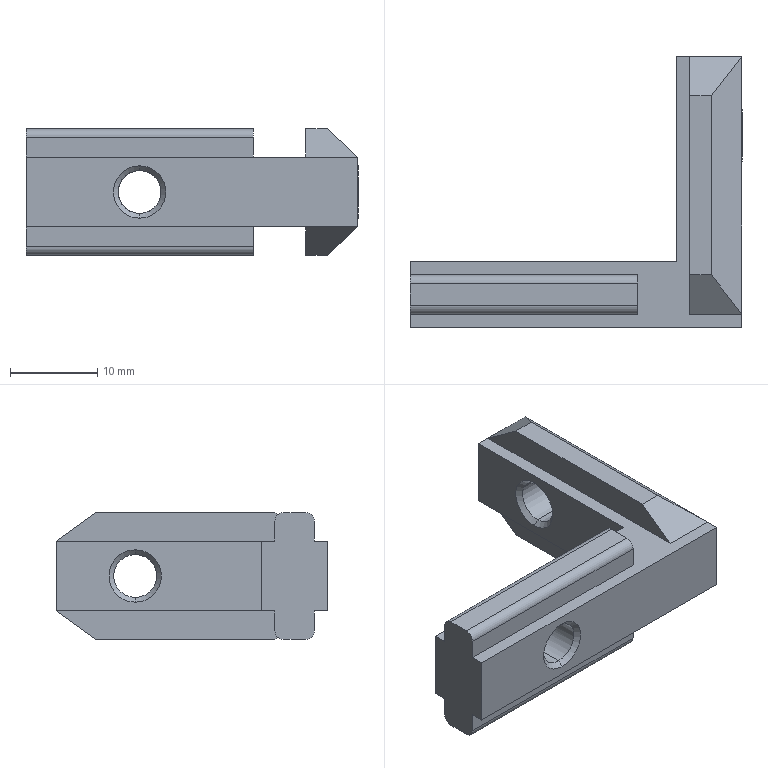Part | SolidWorks | features BaseBody 1 | 1 solid | 42 faces | box 38 x 31 x 14.5 mm | volume 4841 mm3 | plane 26 | cone 8 | cylinder 8 | commonest cylinder face diameters 2 x4 4.917 x4
STEP:
#1=CARTESIAN_POINT('',(12.,0.5415,2.458));
#2=VERTEX_POINT('',#1);
#3=CARTESIAN_POINT('',(12.,0.5415,-2.458));
#4=VERTEX_POINT('',#3);
#5=CARTESIAN_POINT('',(12.,0.5415,0.));
#6=DIRECTION('',(0.,-1.,0.));
#7=DIRECTION('',(0.,0.,-1.));
#8=AXIS2_PLACEMENT_3D('',#5,#6,#7);
#9=CIRCLE('',#8,2.458);
#10=EDGE_CURVE('',#2,#4,#9,.T.);
#11=ORIENTED_EDGE('',*,*,#10,.F.);
#12=CARTESIAN_POINT('',(12.,0.,3.));
#13=VERTEX_POINT('',#12);
#14=CARTESIAN_POINT('',(12.,0.,3.));
#15=DIRECTION('',(0.,-0.7071,0.7071));
#16=VECTOR('',#15,1000.);
#17=LINE('',#14,#16);
#18=EDGE_CURVE('',#2,#13,#17,.T.);
#19=ORIENTED_EDGE('',*,*,#18,.T.);
#20=CARTESIAN_POINT('',(12.,0.,-3.));
#21=VERTEX_POINT('',#20);
#22=CARTESIAN_POINT('',(12.,0.,0.));
#23=DIRECTION('',(0.,-1.,0.));
#24=DIRECTION('',(0.,0.,-1.));
#25=AXIS2_PLACEMENT_3D('',#22,#23,#24);
#26=CIRCLE('',#25,3.);
#27=EDGE_CURVE('',#13,#21,#26,.T.);
#28=ORIENTED_EDGE('',*,*,#27,.T.);
#29=CARTESIAN_POINT('',(12.,0.,-3.));
#30=DIRECTION('',(0.,-0.7071,-0.7071));
#31=VECTOR('',#30,1000.);
#32=LINE('',#29,#31);
#33=EDGE_CURVE('',#4,#21,#32,.T.);
#34=ORIENTED_EDGE('',*,*,#33,.F.);
#35=EDGE_LOOP('',(#11,#19,#28,#34));
#36=FACE_OUTER_BOUND('',#35,.T.);
#37=CARTESIAN_POINT('',(12.,0.,0.));
#38=DIRECTION('',(0.,-1.,0.));
#39=DIRECTION('',(0.,0.,-1.));
#40=AXIS2_PLACEMENT_3D('',#37,#38,#39);
#41=CONICAL_SURFACE('',#40,3.,0.7854);
#42=ADVANCED_FACE('',(#36),#41,.F.);
#43=CARTESIAN_POINT('',(36.458,22.,2.458));
#44=VERTEX_POINT('',#43);
#45=CARTESIAN_POINT('',(36.458,22.,-2.458));
#46=VERTEX_POINT('',#45);
#47=CARTESIAN_POINT('',(36.458,22.,0.));
#48=DIRECTION('',(1.,0.,0.));
#49=DIRECTION('',(0.,0.,-1.));
#50=AXIS2_PLACEMENT_3D('',#47,#48,#49);
#51=CIRCLE('',#50,2.458);
#52=EDGE_CURVE('',#44,#46,#51,.T.);
#53=ORIENTED_EDGE('',*,*,#52,.F.);
#54=CARTESIAN_POINT('',(37.,22.,3.));
#55=VERTEX_POINT('',#54);
#56=CARTESIAN_POINT('',(37.,22.,3.));
#57=DIRECTION('',(0.7071,0.,0.7071));
#58=VECTOR('',#57,1000.);
#59=LINE('',#56,#58);
#60=EDGE_CURVE('',#44,#55,#59,.T.);
#61=ORIENTED_EDGE('',*,*,#60,.T.);
#62=CARTESIAN_POINT('',(37.,22.,-3.));
#63=VERTEX_POINT('',#62);
#64=CARTESIAN_POINT('',(37.,22.,0.));
#65=DIRECTION('',(1.,0.,0.));
#66=DIRECTION('',(0.,0.,-1.));
#67=AXIS2_PLACEMENT_3D('',#64,#65,#66);
#68=CIRCLE('',#67,3.);
#69=EDGE_CURVE('',#55,#63,#68,.T.);
#70=ORIENTED_EDGE('',*,*,#69,.T.);
#71=CARTESIAN_POINT('',(37.,22.,-3.));
#72=DIRECTION('',(0.7071,0.,-0.7071));
#73=VECTOR('',#72,1000.);
#74=LINE('',#71,#73);
#75=EDGE_CURVE('',#46,#63,#74,.T.);
#76=ORIENTED_EDGE('',*,*,#75,.F.);
#77=EDGE_LOOP('',(#53,#61,#70,#76));
#78=FACE_OUTER_BOUND('',#77,.T.);
#79=CARTESIAN_POINT('',(37.,22.,0.));
#80=DIRECTION('',(1.,0.,0.));
#81=DIRECTION('',(0.,0.,-1.));
#82=AXIS2_PLACEMENT_3D('',#79,#80,#81);
#83=CONICAL_SURFACE('',#82,3.,0.7854);
#84=ADVANCED_FACE('',(#78),#83,.F.);
#85=ORIENTED_EDGE('',*,*,#10,.T.);
#86=CARTESIAN_POINT('',(12.,6.958,-2.458));
#87=VERTEX_POINT('',#86);
#88=CARTESIAN_POINT('',(12.,0.,-2.458));
#89=DIRECTION('',(0.,1.,0.));
#90=VECTOR('',#89,1000.);
#91=LINE('',#88,#90);
#92=EDGE_CURVE('',#4,#87,#91,.T.);
#93=ORIENTED_EDGE('',*,*,#92,.T.);
#94=CARTESIAN_POINT('',(9.542,6.958,0.));
#95=VERTEX_POINT('',#94);
#96=CARTESIAN_POINT('',(12.,6.958,0.));
#97=DIRECTION('',(0.,-1.,0.));
#98=DIRECTION('',(0.,0.,1.));
#99=AXIS2_PLACEMENT_3D('',#96,#97,#98);
#100=CIRCLE('',#99,2.458);
#101=EDGE_CURVE('',#95,#87,#100,.T.);
#102=ORIENTED_EDGE('',*,*,#101,.F.);
#103=CARTESIAN_POINT('',(12.,6.958,2.458));
#104=VERTEX_POINT('',#103);
#105=CARTESIAN_POINT('',(12.,6.958,0.));
#106=DIRECTION('',(0.,-1.,0.));
#107=DIRECTION('',(0.,0.,1.));
#108=AXIS2_PLACEMENT_3D('',#105,#106,#107);
#109=CIRCLE('',#108,2.458);
#110=EDGE_CURVE('',#104,#95,#109,.T.);
#111=ORIENTED_EDGE('',*,*,#110,.F.);
#112=CARTESIAN_POINT('',(12.,0.,2.458));
#113=DIRECTION('',(0.,1.,0.));
#114=VECTOR('',#113,1000.);
#115=LINE('',#112,#114);
#116=EDGE_CURVE('',#2,#104,#115,.T.);
#117=ORIENTED_EDGE('',*,*,#116,.F.);
#118=EDGE_LOOP('',(#85,#93,#102,#111,#117));
#119=FACE_OUTER_BOUND('',#118,.T.);
#120=CARTESIAN_POINT('',(12.,0.,0.));
#121=DIRECTION('',(0.,1.,0.));
#122=DIRECTION('',(0.,0.,1.));
#123=AXIS2_PLACEMENT_3D('',#120,#121,#122);
#124=CYLINDRICAL_SURFACE('',#123,2.458);
#125=ADVANCED_FACE('',(#119),#124,.F.);
#126=ORIENTED_EDGE('',*,*,#101,.T.);
#127=CARTESIAN_POINT('',(14.458,6.958,0.));
#128=VERTEX_POINT('',#127);
#129=CARTESIAN_POINT('',(12.,6.958,0.));
#130=DIRECTION('',(0.,-1.,0.));
#131=DIRECTION('',(0.,0.,1.));
#132=AXIS2_PLACEMENT_3D('',#129,#130,#131);
#133=CIRCLE('',#132,2.458);
#134=EDGE_CURVE('',#87,#128,#133,.T.);
#135=ORIENTED_EDGE('',*,*,#134,.T.);
#136=CARTESIAN_POINT('',(15.,7.5,0.));
#137=VERTEX_POINT('',#136);
#138=CARTESIAN_POINT('',(15.,7.5,0.));
#139=DIRECTION('',(0.7071,0.7071,0.));
#140=VECTOR('',#139,1000.);
#141=LINE('',#138,#140);
#142=EDGE_CURVE('',#128,#137,#141,.T.);
#143=ORIENTED_EDGE('',*,*,#142,.T.);
#144=CARTESIAN_POINT('',(9.,7.5,0.));
#145=VERTEX_POINT('',#144);
#146=CARTESIAN_POINT('',(12.,7.5,0.));
#147=DIRECTION('',(0.,1.,0.));
#148=DIRECTION('',(-1.,0.,0.));
#149=AXIS2_PLACEMENT_3D('',#146,#147,#148);
#150=CIRCLE('',#149,3.);
#151=EDGE_CURVE('',#137,#145,#150,.T.);
#152=ORIENTED_EDGE('',*,*,#151,.T.);
#153=CARTESIAN_POINT('',(9.,7.5,0.));
#154=DIRECTION('',(-0.7071,0.7071,0.));
#155=VECTOR('',#154,1000.);
#156=LINE('',#153,#155);
#157=EDGE_CURVE('',#95,#145,#156,.T.);
#158=ORIENTED_EDGE('',*,*,#157,.F.);
#159=EDGE_LOOP('',(#126,#135,#143,#152,#158));
#160=FACE_OUTER_BOUND('',#159,.T.);
#161=CARTESIAN_POINT('',(12.,7.5,0.));
#162=DIRECTION('',(0.,1.,0.));
#163=DIRECTION('',(-1.,0.,0.));
#164=AXIS2_PLACEMENT_3D('',#161,#162,#163);
#165=CONICAL_SURFACE('',#164,3.,0.7854);
#166=ADVANCED_FACE('',(#160),#165,.F.);
#167=CARTESIAN_POINT('',(30.041,22.,-2.458));
#168=VERTEX_POINT('',#167);
#169=CARTESIAN_POINT('',(30.041,22.,2.458));
#170=VERTEX_POINT('',#169);
#171=CARTESIAN_POINT('',(30.041,22.,0.));
#172=DIRECTION('',(-1.,0.,0.));
#173=DIRECTION('',(0.,0.,1.));
#174=AXIS2_PLACEMENT_3D('',#171,#172,#173);
#175=CIRCLE('',#174,2.458);
#176=EDGE_CURVE('',#168,#170,#175,.T.);
#177=ORIENTED_EDGE('',*,*,#176,.F.);
#178=CARTESIAN_POINT('',(29.5,22.,-3.));
#179=VERTEX_POINT('',#178);
#180=CARTESIAN_POINT('',(29.5,22.,-3.));
#181=DIRECTION('',(-0.7071,0.,-0.7071));
#182=VECTOR('',#181,1000.);
#183=LINE('',#180,#182);
#184=EDGE_CURVE('',#168,#179,#183,.T.);
#185=ORIENTED_EDGE('',*,*,#184,.T.);
#186=CARTESIAN_POINT('',(29.5,22.,3.));
#187=VERTEX_POINT('',#186);
#188=CARTESIAN_POINT('',(29.5,22.,0.));
#189=DIRECTION('',(-1.,0.,0.));
#190=DIRECTION('',(0.,0.,1.));
#191=AXIS2_PLACEMENT_3D('',#188,#189,#190);
#192=CIRCLE('',#191,3.);
#193=EDGE_CURVE('',#179,#187,#192,.T.);
#194=ORIENTED_EDGE('',*,*,#193,.T.);
#195=CARTESIAN_POINT('',(29.5,22.,3.));
#196=DIRECTION('',(-0.7071,0.,0.7071));
#197=VECTOR('',#196,1000.);
#198=LINE('',#195,#197);
#199=EDGE_CURVE('',#170,#187,#198,.T.);
#200=ORIENTED_EDGE('',*,*,#199,.F.);
#201=EDGE_LOOP('',(#177,#185,#194,#200));
#202=FACE_OUTER_BOUND('',#201,.T.);
#203=CARTESIAN_POINT('',(29.5,22.,0.));
#204=DIRECTION('',(-1.,0.,0.));
#205=DIRECTION('',(0.,0.,1.));
#206=AXIS2_PLACEMENT_3D('',#203,#204,#205);
#207=CONICAL_SURFACE('',#206,3.,0.7854);
#208=ADVANCED_FACE('',(#202),#207,.F.);
#209=ORIENTED_EDGE('',*,*,#52,.T.);
#210=CARTESIAN_POINT('',(37.,22.,-2.458));
#211=DIRECTION('',(-1.,0.,0.));
#212=VECTOR('',#211,1000.);
#213=LINE('',#210,#212);
#214=EDGE_CURVE('',#46,#168,#213,.T.);
#215=ORIENTED_EDGE('',*,*,#214,.T.);
#216=ORIENTED_EDGE('',*,*,#176,.T.);
#217=CARTESIAN_POINT('',(37.,22.,2.458));
#218=DIRECTION('',(-1.,0.,0.));
#219=VECTOR('',#218,1000.);
#220=LINE('',#217,#219);
#221=EDGE_CURVE('',#44,#170,#220,.T.);
#222=ORIENTED_EDGE('',*,*,#221,.F.);
#223=EDGE_LOOP('',(#209,#215,#216,#222));
#224=FACE_OUTER_BOUND('',#223,.T.);
#225=CARTESIAN_POINT('',(37.,22.,0.));
#226=DIRECTION('',(-1.,0.,0.));
#227=DIRECTION('',(0.,0.,1.));
#228=AXIS2_PLACEMENT_3D('',#225,#226,#227);
#229=CYLINDRICAL_SURFACE('',#228,2.458);
#230=ADVANCED_FACE('',(#224),#229,.F.);
#231=CARTESIAN_POINT('',(37.,0.,4.));
#232=VERTEX_POINT('',#231);
#233=CARTESIAN_POINT('',(37.,0.,-4.));
#234=VERTEX_POINT('',#233);
#235=CARTESIAN_POINT('',(37.,0.,4.));
#236=DIRECTION('',(0.,0.,-1.));
#237=VECTOR('',#236,1000.);
#238=LINE('',#235,#237);
#239=EDGE_CURVE('',#232,#234,#238,.T.);
#240=ORIENTED_EDGE('',*,*,#239,.F.);
#241=CARTESIAN_POINT('',(-1.,0.,4.));
#242=VERTEX_POINT('',#241);
#243=CARTESIAN_POINT('',(-1.,0.,4.));
#244=DIRECTION('',(1.,0.,0.));
#245=VECTOR('',#244,1000.);
#246=LINE('',#243,#245);
#247=EDGE_CURVE('',#242,#232,#246,.T.);
#248=ORIENTED_EDGE('',*,*,#247,.F.);
#249=CARTESIAN_POINT('',(-1.,0.,-4.));
#250=VERTEX_POINT('',#249);
#251=CARTESIAN_POINT('',(-1.,0.,4.));
#252=DIRECTION('',(0.,0.,1.));
#253=VECTOR('',#252,1000.);
#254=LINE('',#251,#253);
#255=EDGE_CURVE('',#250,#242,#254,.T.);
#256=ORIENTED_EDGE('',*,*,#255,.F.);
#257=CARTESIAN_POINT('',(-1.,0.,-4.));
#258=DIRECTION('',(-1.,0.,0.));
#259=VECTOR('',#258,1000.);
#260=LINE('',#257,#259);
#261=EDGE_CURVE('',#234,#250,#260,.T.);
#262=ORIENTED_EDGE('',*,*,#261,.F.);
#263=EDGE_LOOP('',(#240,#248,#256,#262));
#264=FACE_OUTER_BOUND('',#263,.T.);
#265=CARTESIAN_POINT('',(12.,0.,0.));
#266=DIRECTION('',(0.,-1.,0.));
#267=DIRECTION('',(0.,0.,-1.));
#268=AXIS2_PLACEMENT_3D('',#265,#266,#267);
#269=CIRCLE('',#268,3.);
#270=EDGE_CURVE('',#21,#13,#269,.T.);
#271=ORIENTED_EDGE('',*,*,#270,.F.);
#272=ORIENTED_EDGE('',*,*,#27,.F.);
#273=EDGE_LOOP('',(#271,#272));
#274=FACE_BOUND('',#273,.T.);
#275=CARTESIAN_POINT('',(-1.,0.,4.));
#276=DIRECTION('',(0.,1.,0.));
#277=DIRECTION('',(0.,0.,1.));
#278=AXIS2_PLACEMENT_3D('',#275,#276,#277);
#279=PLANE('',#278);
#280=ADVANCED_FACE('',(#264,#274),#279,.F.);
#281=ORIENTED_EDGE('',*,*,#261,.T.);
#282=CARTESIAN_POINT('',(-1.,1.5,-4.));
#283=VERTEX_POINT('',#282);
#284=CARTESIAN_POINT('',(-1.,0.,-4.));
#285=DIRECTION('',(0.,-1.,0.));
#286=VECTOR('',#285,1000.);
#287=LINE('',#284,#286);
#288=EDGE_CURVE('',#283,#250,#287,.T.);
#289=ORIENTED_EDGE('',*,*,#288,.F.);
#290=CARTESIAN_POINT('',(25.,1.5,-4.));
#291=VERTEX_POINT('',#290);
#292=CARTESIAN_POINT('',(0.,1.5,-4.));
#293=DIRECTION('',(-1.,0.,0.));
#294=VECTOR('',#293,1000.);
#295=LINE('',#292,#294);
#296=EDGE_CURVE('',#291,#283,#295,.T.);
#297=ORIENTED_EDGE('',*,*,#296,.F.);
#298=CARTESIAN_POINT('',(25.,6.,-4.));
#299=VERTEX_POINT('',#298);
#300=CARTESIAN_POINT('',(25.,0.,-4.));
#301=DIRECTION('',(0.,-1.,0.));
#302=VECTOR('',#301,1000.);
#303=LINE('',#300,#302);
#304=EDGE_CURVE('',#299,#291,#303,.T.);
#305=ORIENTED_EDGE('',*,*,#304,.F.);
#306=CARTESIAN_POINT('',(-1.,6.,-4.));
#307=VERTEX_POINT('',#306);
#308=CARTESIAN_POINT('',(0.,6.,-4.));
#309=DIRECTION('',(1.,0.,0.));
#310=VECTOR('',#309,1000.);
#311=LINE('',#308,#310);
#312=EDGE_CURVE('',#307,#299,#311,.T.);
#313=ORIENTED_EDGE('',*,*,#312,.F.);
#314=CARTESIAN_POINT('',(-1.,7.5,-4.));
#315=VERTEX_POINT('',#314);
#316=CARTESIAN_POINT('',(-1.,0.,-4.));
#317=DIRECTION('',(0.,-1.,0.));
#318=VECTOR('',#317,1000.);
#319=LINE('',#316,#318);
#320=EDGE_CURVE('',#315,#307,#319,.T.);
#321=ORIENTED_EDGE('',*,*,#320,.F.);
#322=CARTESIAN_POINT('',(29.5,7.5,-4.));
#323=VERTEX_POINT('',#322);
#324=CARTESIAN_POINT('',(0.,7.5,-4.));
#325=DIRECTION('',(-1.,0.,0.));
#326=VECTOR('',#325,1000.);
#327=LINE('',#324,#326);
#328=EDGE_CURVE('',#323,#315,#327,.T.);
#329=ORIENTED_EDGE('',*,*,#328,.F.);
#330=CARTESIAN_POINT('',(29.5,31.,-4.));
#331=VERTEX_POINT('',#330);
#332=CARTESIAN_POINT('',(29.5,0.,-4.));
#333=DIRECTION('',(0.,-1.,0.));
#334=VECTOR('',#333,1000.);
#335=LINE('',#332,#334);
#336=EDGE_CURVE('',#331,#323,#335,.T.);
#337=ORIENTED_EDGE('',*,*,#336,.F.);
#338=CARTESIAN_POINT('',(31.,31.,-4.));
#339=VERTEX_POINT('',#338);
#340=CARTESIAN_POINT('',(37.,31.,-4.));
#341=DIRECTION('',(1.,0.,0.));
#342=VECTOR('',#341,1000.);
#343=LINE('',#340,#342);
#344=EDGE_CURVE('',#331,#339,#343,.T.);
#345=ORIENTED_EDGE('',*,*,#344,.T.);
#346=CARTESIAN_POINT('',(31.,1.5,-4.));
#347=VERTEX_POINT('',#346);
#348=CARTESIAN_POINT('',(31.,0.,-4.));
#349=DIRECTION('',(0.,1.,0.));
#350=VECTOR('',#349,1000.);
#351=LINE('',#348,#350);
#352=EDGE_CURVE('',#347,#339,#351,.T.);
#353=ORIENTED_EDGE('',*,*,#352,.F.);
#354=CARTESIAN_POINT('',(37.,1.5,-4.));
#355=VERTEX_POINT('',#354);
#356=CARTESIAN_POINT('',(0.,1.5,-4.));
#357=DIRECTION('',(-1.,0.,0.));
#358=VECTOR('',#357,1000.);
#359=LINE('',#356,#358);
#360=EDGE_CURVE('',#355,#347,#359,.T.);
#361=ORIENTED_EDGE('',*,*,#360,.F.);
#362=CARTESIAN_POINT('',(37.,0.,-4.));
#363=DIRECTION('',(0.,1.,0.));
#364=VECTOR('',#363,1000.);
#365=LINE('',#362,#364);
#366=EDGE_CURVE('',#234,#355,#365,.T.);
#367=ORIENTED_EDGE('',*,*,#366,.F.);
#368=EDGE_LOOP('',(#281,#289,#297,#305,#313,#321,#329,#337,#345,#353,#361,#367));
#369=FACE_OUTER_BOUND('',#368,.T.);
#370=CARTESIAN_POINT('',(0.,0.,-4.));
#371=DIRECTION('',(0.,0.,1.));
#372=DIRECTION('',(1.,0.,0.));
#373=AXIS2_PLACEMENT_3D('',#370,#371,#372);
#374=PLANE('',#373);
#375=ADVANCED_FACE('',(#369),#374,.F.);
#376=CARTESIAN_POINT('',(37.,31.,-4.));
#377=VERTEX_POINT('',#376);
#378=CARTESIAN_POINT('',(37.,0.,-4.));
#379=DIRECTION('',(0.,-1.,0.));
#380=VECTOR('',#379,1000.);
#381=LINE('',#378,#380);
#382=EDGE_CURVE('',#377,#355,#381,.T.);
#383=ORIENTED_EDGE('',*,*,#382,.F.);
#384=CARTESIAN_POINT('',(37.,31.,4.));
#385=VERTEX_POINT('',#384);
#386=CARTESIAN_POINT('',(37.,31.,4.));
#387=DIRECTION('',(0.,0.,-1.));
#388=VECTOR('',#387,1000.);
#389=LINE('',#386,#388);
#390=EDGE_CURVE('',#385,#377,#389,.T.);
#391=ORIENTED_EDGE('',*,*,#390,.F.);
#392=CARTESIAN_POINT('',(37.,1.5,4.));
#393=VERTEX_POINT('',#392);
#394=CARTESIAN_POINT('',(37.,0.,4.));
#395=DIRECTION('',(0.,1.,0.));
#396=VECTOR('',#395,1000.);
#397=LINE('',#394,#396);
#398=EDGE_CURVE('',#393,#385,#397,.T.);
#399=ORIENTED_EDGE('',*,*,#398,.F.);
#400=CARTESIAN_POINT('',(37.,0.,4.));
#401=DIRECTION('',(0.,1.,0.));
#402=VECTOR('',#401,1000.);
#403=LINE('',#400,#402);
#404=EDGE_CURVE('',#232,#393,#403,.T.);
#405=ORIENTED_EDGE('',*,*,#404,.F.);
#406=ORIENTED_EDGE('',*,*,#239,.T.);
#407=ORIENTED_EDGE('',*,*,#366,.T.);
#408=EDGE_LOOP('',(#383,#391,#399,#405,#406,#407));
#409=FACE_OUTER_BOUND('',#408,.T.);
#410=CARTESIAN_POINT('',(37.,22.,0.));
#411=DIRECTION('',(1.,0.,0.));
#412=DIRECTION('',(0.,0.,-1.));
#413=AXIS2_PLACEMENT_3D('',#410,#411,#412);
#414=CIRCLE('',#413,3.);
#415=EDGE_CURVE('',#63,#55,#414,.T.);
#416=ORIENTED_EDGE('',*,*,#415,.F.);
#417=ORIENTED_EDGE('',*,*,#69,.F.);
#418=EDGE_LOOP('',(#416,#417));
#419=FACE_BOUND('',#418,.T.);
#420=CARTESIAN_POINT('',(37.,0.,4.));
#421=DIRECTION('',(-1.,0.,0.));
#422=DIRECTION('',(0.,0.,1.));
#423=AXIS2_PLACEMENT_3D('',#420,#421,#422);
#424=PLANE('',#423);
#425=ADVANCED_FACE('',(#409,#419),#424,.F.);
#426=CARTESIAN_POINT('',(25.,1.5,4.));
#427=VERTEX_POINT('',#426);
#428=CARTESIAN_POINT('',(-1.,1.5,4.));
#429=VERTEX_POINT('',#428);
#430=CARTESIAN_POINT('',(0.,1.5,4.));
#431=DIRECTION('',(-1.,0.,0.));
#432=VECTOR('',#431,1000.);
#433=LINE('',#430,#432);
#434=EDGE_CURVE('',#427,#429,#433,.T.);
#435=ORIENTED_EDGE('',*,*,#434,.T.);
#436=CARTESIAN_POINT('',(-1.,0.,4.));
#437=DIRECTION('',(0.,-1.,0.));
#438=VECTOR('',#437,1000.);
#439=LINE('',#436,#438);
#440=EDGE_CURVE('',#429,#242,#439,.T.);
#441=ORIENTED_EDGE('',*,*,#440,.T.);
#442=ORIENTED_EDGE('',*,*,#247,.T.);
#443=ORIENTED_EDGE('',*,*,#404,.T.);
#444=CARTESIAN_POINT('',(31.,1.5,4.));
#445=VERTEX_POINT('',#444);
#446=CARTESIAN_POINT('',(0.,1.5,4.));
#447=DIRECTION('',(-1.,0.,0.));
#448=VECTOR('',#447,1000.);
#449=LINE('',#446,#448);
#450=EDGE_CURVE('',#393,#445,#449,.T.);
#451=ORIENTED_EDGE('',*,*,#450,.T.);
#452=CARTESIAN_POINT('',(31.,31.,4.));
#453=VERTEX_POINT('',#452);
#454=CARTESIAN_POINT('',(31.,0.,4.));
#455=DIRECTION('',(0.,1.,0.));
#456=VECTOR('',#455,1000.);
#457=LINE('',#454,#456);
#458=EDGE_CURVE('',#445,#453,#457,.T.);
#459=ORIENTED_EDGE('',*,*,#458,.T.);
#460=CARTESIAN_POINT('',(29.5,31.,4.));
#461=VERTEX_POINT('',#460);
#462=CARTESIAN_POINT('',(0.,31.,4.));
#463=DIRECTION('',(-1.,0.,0.));
#464=VECTOR('',#463,1000.);
#465=LINE('',#462,#464);
#466=EDGE_CURVE('',#453,#461,#465,.T.);
#467=ORIENTED_EDGE('',*,*,#466,.T.);
#468=CARTESIAN_POINT('',(29.5,7.5,4.));
#469=VERTEX_POINT('',#468);
#470=CARTESIAN_POINT('',(29.5,0.,4.));
#471=DIRECTION('',(0.,-1.,0.));
#472=VECTOR('',#471,1000.);
#473=LINE('',#470,#472);
#474=EDGE_CURVE('',#461,#469,#473,.T.);
#475=ORIENTED_EDGE('',*,*,#474,.T.);
#476=CARTESIAN_POINT('',(-1.,7.5,4.));
#477=VERTEX_POINT('',#476);
#478=CARTESIAN_POINT('',(0.,7.5,4.));
#479=DIRECTION('',(-1.,0.,0.));
#480=VECTOR('',#479,1000.);
#481=LINE('',#478,#480);
#482=EDGE_CURVE('',#469,#477,#481,.T.);
#483=ORIENTED_EDGE('',*,*,#482,.T.);
#484=CARTESIAN_POINT('',(-1.,6.,4.));
#485=VERTEX_POINT('',#484);
#486=CARTESIAN_POINT('',(-1.,0.,4.));
#487=DIRECTION('',(0.,-1.,0.));
#488=VECTOR('',#487,1000.);
#489=LINE('',#486,#488);
#490=EDGE_CURVE('',#477,#485,#489,.T.);
#491=ORIENTED_EDGE('',*,*,#490,.T.);
#492=CARTESIAN_POINT('',(25.,6.,4.));
#493=VERTEX_POINT('',#492);
#494=CARTESIAN_POINT('',(0.,6.,4.));
#495=DIRECTION('',(1.,0.,0.));
#496=VECTOR('',#495,1000.);
#497=LINE('',#494,#496);
#498=EDGE_CURVE('',#485,#493,#497,.T.);
#499=ORIENTED_EDGE('',*,*,#498,.T.);
#500=CARTESIAN_POINT('',(25.,0.,4.));
#501=DIRECTION('',(0.,-1.,0.));
#502=VECTOR('',#501,1000.);
#503=LINE('',#500,#502);
#504=EDGE_CURVE('',#493,#427,#503,.T.);
#505=ORIENTED_EDGE('',*,*,#504,.T.);
#506=EDGE_LOOP('',(#435,#441,#442,#443,#451,#459,#467,#475,#483,#491,#499,#505));
#507=FACE_OUTER_BOUND('',#506,.T.);
#508=CARTESIAN_POINT('',(0.,0.,4.));
#509=DIRECTION('',(0.,0.,1.));
#510=DIRECTION('',(1.,0.,0.));
#511=AXIS2_PLACEMENT_3D('',#508,#509,#510);
#512=PLANE('',#511);
#513=ADVANCED_FACE('',(#507),#512,.T.);
#514=CARTESIAN_POINT('',(-1.,6.,-6.25));
#515=VERTEX_POINT('',#514);
#516=CARTESIAN_POINT('',(-1.,6.,4.));
#517=DIRECTION('',(0.,0.,1.));
#518=VECTOR('',#517,1000.);
#519=LINE('',#516,#518);
#520=EDGE_CURVE('',#515,#307,#519,.T.);
#521=ORIENTED_EDGE('',*,*,#520,.F.);
#522=CARTESIAN_POINT('',(-1.,5.,-7.25));
#523=VERTEX_POINT('',#522);
#524=CARTESIAN_POINT('',(-1.,5.,-6.25));
#525=DIRECTION('',(1.,0.,0.));
#526=DIRECTION('',(0.,0.,-1.));
#527=AXIS2_PLACEMENT_3D('',#524,#525,#526);
#528=CIRCLE('',#527,1.);
#529=EDGE_CURVE('',#523,#515,#528,.T.);
#530=ORIENTED_EDGE('',*,*,#529,.F.);
#531=CARTESIAN_POINT('',(-1.,2.5,-7.25));
#532=VERTEX_POINT('',#531);
#533=CARTESIAN_POINT('',(-1.,7.5,-7.25));
#534=DIRECTION('',(0.,1.,0.));
#535=VECTOR('',#534,1000.);
#536=LINE('',#533,#535);
#537=EDGE_CURVE('',#532,#523,#536,.T.);
#538=ORIENTED_EDGE('',*,*,#537,.F.);
#539=CARTESIAN_POINT('',(-1.,1.5,-6.25));
#540=VERTEX_POINT('',#539);
#541=CARTESIAN_POINT('',(-1.,2.5,-6.25));
#542=DIRECTION('',(1.,0.,0.));
#543=DIRECTION('',(0.,0.,-1.));
#544=AXIS2_PLACEMENT_3D('',#541,#542,#543);
#545=CIRCLE('',#544,1.);
#546=EDGE_CURVE('',#540,#532,#545,.T.);
#547=ORIENTED_EDGE('',*,*,#546,.F.);
#548=CARTESIAN_POINT('',(-1.,1.5,4.));
#549=DIRECTION('',(0.,0.,-1.));
#550=VECTOR('',#549,1000.);
#551=LINE('',#548,#550);
#552=EDGE_CURVE('',#283,#540,#551,.T.);
#553=ORIENTED_EDGE('',*,*,#552,.F.);
#554=ORIENTED_EDGE('',*,*,#288,.T.);
#555=ORIENTED_EDGE('',*,*,#255,.T.);
#556=ORIENTED_EDGE('',*,*,#440,.F.);
#557=CARTESIAN_POINT('',(-1.,1.5,6.25));
#558=VERTEX_POINT('',#557);
#559=CARTESIAN_POINT('',(-1.,1.5,4.));
#560=DIRECTION('',(0.,0.,-1.));
#561=VECTOR('',#560,1000.);
#562=LINE('',#559,#561);
#563=EDGE_CURVE('',#558,#429,#562,.T.);
#564=ORIENTED_EDGE('',*,*,#563,.F.);
#565=CARTESIAN_POINT('',(-1.,2.5,7.25));
#566=VERTEX_POINT('',#565);
#567=CARTESIAN_POINT('',(-1.,2.5,6.25));
#568=DIRECTION('',(1.,0.,0.));
#569=DIRECTION('',(0.,0.,-1.));
#570=AXIS2_PLACEMENT_3D('',#567,#568,#569);
#571=CIRCLE('',#570,1.);
#572=EDGE_CURVE('',#566,#558,#571,.T.);
#573=ORIENTED_EDGE('',*,*,#572,.F.);
#574=CARTESIAN_POINT('',(-1.,5.,7.25));
#575=VERTEX_POINT('',#574);
#576=CARTESIAN_POINT('',(-1.,7.5,7.25));
#577=DIRECTION('',(0.,-1.,0.));
#578=VECTOR('',#577,1000.);
#579=LINE('',#576,#578);
#580=EDGE_CURVE('',#575,#566,#579,.T.);
#581=ORIENTED_EDGE('',*,*,#580,.F.);
#582=CARTESIAN_POINT('',(-1.,6.,6.25));
#583=VERTEX_POINT('',#582);
#584=CARTESIAN_POINT('',(-1.,5.,6.25));
#585=DIRECTION('',(1.,0.,0.));
#586=DIRECTION('',(0.,0.,-1.));
#587=AXIS2_PLACEMENT_3D('',#584,#585,#586);
#588=CIRCLE('',#587,1.);
#589=EDGE_CURVE('',#583,#575,#588,.T.);
#590=ORIENTED_EDGE('',*,*,#589,.F.);
#591=CARTESIAN_POINT('',(-1.,6.,4.));
#592=DIRECTION('',(0.,0.,1.));
#593=VECTOR('',#592,1000.);
#594=LINE('',#591,#593);
#595=EDGE_CURVE('',#485,#583,#594,.T.);
#596=ORIENTED_EDGE('',*,*,#595,.F.);
#597=ORIENTED_EDGE('',*,*,#490,.F.);
#598=CARTESIAN_POINT('',(-1.,7.5,4.));
#599=DIRECTION('',(0.,0.,1.));
#600=VECTOR('',#599,1000.);
#601=LINE('',#598,#600);
#602=EDGE_CURVE('',#315,#477,#601,.T.);
#603=ORIENTED_EDGE('',*,*,#602,.F.);
#604=ORIENTED_EDGE('',*,*,#320,.T.);
#605=EDGE_LOOP('',(#521,#530,#538,#547,#553,#554,#555,#556,#564,#573,#581,#590,#596,#597,#603,#604));
#606=FACE_OUTER_BOUND('',#605,.T.);
#607=CARTESIAN_POINT('',(-1.,7.5,4.));
#608=DIRECTION('',(1.,0.,0.));
#609=DIRECTION('',(0.,0.,-1.));
#610=AXIS2_PLACEMENT_3D('',#607,#608,#609);
#611=PLANE('',#610);
#612=ADVANCED_FACE('',(#606),#611,.F.);
#613=ORIENTED_EDGE('',*,*,#18,.F.);
#614=CARTESIAN_POINT('',(12.,0.5415,0.));
#615=DIRECTION('',(0.,-1.,0.));
#616=DIRECTION('',(0.,0.,-1.));
#617=AXIS2_PLACEMENT_3D('',#614,#615,#616);
#618=CIRCLE('',#617,2.458);
#619=EDGE_CURVE('',#4,#2,#618,.T.);
#620=ORIENTED_EDGE('',*,*,#619,.F.);
#621=ORIENTED_EDGE('',*,*,#33,.T.);
#622=ORIENTED_EDGE('',*,*,#270,.T.);
#623=EDGE_LOOP('',(#613,#620,#621,#622));
#624=FACE_OUTER_BOUND('',#623,.T.);
#625=CARTESIAN_POINT('',(12.,0.,0.));
#626=DIRECTION('',(0.,-1.,0.));
#627=DIRECTION('',(0.,0.,-1.));
#628=AXIS2_PLACEMENT_3D('',#625,#626,#627);
#629=CONICAL_SURFACE('',#628,3.,0.7854);
#630=ADVANCED_FACE('',(#624),#629,.F.);
#631=CARTESIAN_POINT('',(25.,1.5,-6.25));
#632=VERTEX_POINT('',#631);
#633=CARTESIAN_POINT('',(25.,1.5,-6.25));
#634=DIRECTION('',(-1.,0.,0.));
#635=VECTOR('',#634,1000.);
#636=LINE('',#633,#635);
#637=EDGE_CURVE('',#632,#540,#636,.T.);
#638=ORIENTED_EDGE('',*,*,#637,.F.);
#639=CARTESIAN_POINT('',(25.,1.5,-4.));
#640=DIRECTION('',(0.,0.,-1.));
#641=VECTOR('',#640,1000.);
#642=LINE('',#639,#641);
#643=EDGE_CURVE('',#291,#632,#642,.T.);
#644=ORIENTED_EDGE('',*,*,#643,.F.);
#645=ORIENTED_EDGE('',*,*,#296,.T.);
#646=ORIENTED_EDGE('',*,*,#552,.T.);
#647=EDGE_LOOP('',(#638,#644,#645,#646));
#648=FACE_OUTER_BOUND('',#647,.T.);
#649=CARTESIAN_POINT('',(25.,1.5,-4.));
#650=DIRECTION('',(0.,1.,0.));
#651=DIRECTION('',(0.,0.,1.));
#652=AXIS2_PLACEMENT_3D('',#649,#650,#651);
#653=PLANE('',#652);
#654=ADVANCED_FACE('',(#648),#653,.F.);
#655=CARTESIAN_POINT('',(25.,2.5,-7.25));
#656=VERTEX_POINT('',#655);
#657=CARTESIAN_POINT('',(25.,5.,-7.25));
#658=VERTEX_POINT('',#657);
#659=CARTESIAN_POINT('',(25.,2.5,-7.25));
#660=DIRECTION('',(0.,1.,0.));
#661=VECTOR('',#660,1000.);
#662=LINE('',#659,#661);
#663=EDGE_CURVE('',#656,#658,#662,.T.);
#664=ORIENTED_EDGE('',*,*,#663,.T.);
#665=CARTESIAN_POINT('',(25.,6.,-6.25));
#666=VERTEX_POINT('',#665);
#667=CARTESIAN_POINT('',(25.,5.,-6.25));
#668=DIRECTION('',(-1.,0.,0.));
#669=DIRECTION('',(0.,0.,-1.));
#670=AXIS2_PLACEMENT_3D('',#667,#668,#669);
#671=CIRCLE('',#670,1.);
#672=EDGE_CURVE('',#666,#658,#671,.T.);
#673=ORIENTED_EDGE('',*,*,#672,.F.);
#674=CARTESIAN_POINT('',(25.,6.,-6.25));
#675=DIRECTION('',(0.,0.,1.));
#676=VECTOR('',#675,1000.);
#677=LINE('',#674,#676);
#678=EDGE_CURVE('',#666,#299,#677,.T.);
#679=ORIENTED_EDGE('',*,*,#678,.T.);
#680=ORIENTED_EDGE('',*,*,#304,.T.);
#681=ORIENTED_EDGE('',*,*,#643,.T.);
#682=CARTESIAN_POINT('',(25.,2.5,-6.25));
#683=DIRECTION('',(1.,0.,0.));
#684=DIRECTION('',(0.,0.,-1.));
#685=AXIS2_PLACEMENT_3D('',#682,#683,#684);
#686=CIRCLE('',#685,1.);
#687=EDGE_CURVE('',#632,#656,#686,.T.);
#688=ORIENTED_EDGE('',*,*,#687,.T.);
#689=EDGE_LOOP('',(#664,#673,#679,#680,#681,#688));
#690=FACE_OUTER_BOUND('',#689,.T.);
#691=CARTESIAN_POINT('',(25.,2.5,-6.25));
#692=DIRECTION('',(1.,0.,0.));
#693=DIRECTION('',(0.,0.,-1.));
#694=AXIS2_PLACEMENT_3D('',#691,#692,#693);
#695=PLANE('',#694);
#696=ADVANCED_FACE('',(#690),#695,.T.);
#697=ORIENTED_EDGE('',*,*,#312,.T.);
#698=ORIENTED_EDGE('',*,*,#678,.F.);
#699=CARTESIAN_POINT('',(25.,6.,-6.25));
#700=DIRECTION('',(1.,0.,0.));
#701=VECTOR('',#700,1000.);
#702=LINE('',#699,#701);
#703=EDGE_CURVE('',#515,#666,#702,.T.);
#704=ORIENTED_EDGE('',*,*,#703,.F.);
#705=ORIENTED_EDGE('',*,*,#520,.T.);
#706=EDGE_LOOP('',(#697,#698,#704,#705));
#707=FACE_OUTER_BOUND('',#706,.T.);
#708=CARTESIAN_POINT('',(25.,6.,-6.25));
#709=DIRECTION('',(0.,-1.,0.));
#710=DIRECTION('',(0.,0.,-1.));
#711=AXIS2_PLACEMENT_3D('',#708,#709,#710);
#712=PLANE('',#711);
#713=ADVANCED_FACE('',(#707),#712,.F.);
#714=ORIENTED_EDGE('',*,*,#602,.T.);
#715=ORIENTED_EDGE('',*,*,#482,.F.);
#716=CARTESIAN_POINT('',(29.5,7.5,4.));
#717=DIRECTION('',(0.,0.,1.));
#718=VECTOR('',#717,1000.);
#719=LINE('',#716,#718);
#720=EDGE_CURVE('',#323,#469,#719,.T.);
#721=ORIENTED_EDGE('',*,*,#720,.F.);
#722=ORIENTED_EDGE('',*,*,#328,.T.);
#723=EDGE_LOOP('',(#714,#715,#721,#722));
#724=FACE_OUTER_BOUND('',#723,.T.);
#725=CARTESIAN_POINT('',(12.,7.5,0.));
#726=DIRECTION('',(0.,1.,0.));
#727=DIRECTION('',(-1.,0.,0.));
#728=AXIS2_PLACEMENT_3D('',#725,#726,#727);
#729=CIRCLE('',#728,3.);
#730=EDGE_CURVE('',#145,#137,#729,.T.);
#731=ORIENTED_EDGE('',*,*,#730,.F.);
#732=ORIENTED_EDGE('',*,*,#151,.F.);
#733=EDGE_LOOP('',(#731,#732));
#734=FACE_BOUND('',#733,.T.);
#735=CARTESIAN_POINT('',(29.5,7.5,4.));
#736=DIRECTION('',(0.,-1.,0.));
#737=DIRECTION('',(0.,0.,-1.));
#738=AXIS2_PLACEMENT_3D('',#735,#736,#737);
#739=PLANE('',#738);
#740=ADVANCED_FACE('',(#724,#734),#739,.F.);
#741=ORIENTED_EDGE('',*,*,#720,.T.);
#742=ORIENTED_EDGE('',*,*,#474,.F.);
#743=CARTESIAN_POINT('',(29.5,31.,4.));
#744=DIRECTION('',(0.,0.,1.));
#745=VECTOR('',#744,1000.);
#746=LINE('',#743,#745);
#747=EDGE_CURVE('',#331,#461,#746,.T.);
#748=ORIENTED_EDGE('',*,*,#747,.F.);
#749=ORIENTED_EDGE('',*,*,#336,.T.);
#750=EDGE_LOOP('',(#741,#742,#748,#749));
#751=FACE_OUTER_BOUND('',#750,.T.);
#752=CARTESIAN_POINT('',(29.5,22.,0.));
#753=DIRECTION('',(-1.,0.,0.));
#754=DIRECTION('',(0.,0.,1.));
#755=AXIS2_PLACEMENT_3D('',#752,#753,#754);
#756=CIRCLE('',#755,3.);
#757=EDGE_CURVE('',#187,#179,#756,.T.);
#758=ORIENTED_EDGE('',*,*,#757,.F.);
#759=ORIENTED_EDGE('',*,*,#193,.F.);
#760=EDGE_LOOP('',(#758,#759));
#761=FACE_BOUND('',#760,.T.);
#762=CARTESIAN_POINT('',(29.5,31.,4.));
#763=DIRECTION('',(1.,0.,0.));
#764=DIRECTION('',(0.,0.,-1.));
#765=AXIS2_PLACEMENT_3D('',#762,#763,#764);
#766=PLANE('',#765);
#767=ADVANCED_FACE('',(#751,#761),#766,.F.);
#768=ORIENTED_EDGE('',*,*,#352,.T.);
#769=CARTESIAN_POINT('',(31.,26.5,-7.25));
#770=VERTEX_POINT('',#769);
#771=CARTESIAN_POINT('',(31.,26.5,-7.25));
#772=DIRECTION('',(0.,0.8107,0.5855));
#773=VECTOR('',#772,1000.);
#774=LINE('',#771,#773);
#775=EDGE_CURVE('',#770,#339,#774,.T.);
#776=ORIENTED_EDGE('',*,*,#775,.F.);
#777=CARTESIAN_POINT('',(31.,6.,-7.25));
#778=VERTEX_POINT('',#777);
#779=CARTESIAN_POINT('',(31.,31.,-7.25));
#780=DIRECTION('',(0.,1.,0.));
#781=VECTOR('',#780,1000.);
#782=LINE('',#779,#781);
#783=EDGE_CURVE('',#778,#770,#782,.T.);
#784=ORIENTED_EDGE('',*,*,#783,.F.);
#785=CARTESIAN_POINT('',(31.,1.5,-4.));
#786=DIRECTION('',(0.,0.8107,-0.5855));
#787=VECTOR('',#786,1000.);
#788=LINE('',#785,#787);
#789=EDGE_CURVE('',#347,#778,#788,.T.);
#790=ORIENTED_EDGE('',*,*,#789,.F.);
#791=EDGE_LOOP('',(#768,#776,#784,#790));
#792=FACE_OUTER_BOUND('',#791,.T.);
#793=CARTESIAN_POINT('',(31.,31.,-7.25));
#794=DIRECTION('',(1.,0.,0.));
#795=DIRECTION('',(0.,0.,-1.));
#796=AXIS2_PLACEMENT_3D('',#793,#794,#795);
#797=PLANE('',#796);
#798=ADVANCED_FACE('',(#792),#797,.F.);
#799=ORIENTED_EDGE('',*,*,#789,.T.);
#800=CARTESIAN_POINT('',(33.5,6.,-7.25));
#801=VERTEX_POINT('',#800);
#802=CARTESIAN_POINT('',(91.,6.,-7.25));
#803=DIRECTION('',(1.,0.,0.));
#804=VECTOR('',#803,1000.);
#805=LINE('',#802,#804);
#806=EDGE_CURVE('',#778,#801,#805,.T.);
#807=ORIENTED_EDGE('',*,*,#806,.T.);
#808=CARTESIAN_POINT('',(33.5,6.,-7.25));
#809=DIRECTION('',(0.5334,-0.6857,0.4953));
#810=VECTOR('',#809,1000.);
#811=LINE('',#808,#810);
#812=EDGE_CURVE('',#801,#355,#811,.T.);
#813=ORIENTED_EDGE('',*,*,#812,.T.);
#814=ORIENTED_EDGE('',*,*,#360,.T.);
#815=EDGE_LOOP('',(#799,#807,#813,#814));
#816=FACE_OUTER_BOUND('',#815,.T.);
#817=CARTESIAN_POINT('',(91.,6.,-7.25));
#818=DIRECTION('',(0.,-0.5855,-0.8107));
#819=DIRECTION('',(0.,0.8107,-0.5855));
#820=AXIS2_PLACEMENT_3D('',#817,#818,#819);
#821=PLANE('',#820);
#822=ADVANCED_FACE('',(#816),#821,.T.);
#823=CARTESIAN_POINT('',(33.5,26.5,-7.25));
#824=VERTEX_POINT('',#823);
#825=CARTESIAN_POINT('',(33.5,31.,-7.25));
#826=DIRECTION('',(0.,-1.,0.));
#827=VECTOR('',#826,1000.);
#828=LINE('',#825,#827);
#829=EDGE_CURVE('',#824,#801,#828,.T.);
#830=ORIENTED_EDGE('',*,*,#829,.F.);
#831=CARTESIAN_POINT('',(37.,31.,-4.));
#832=DIRECTION('',(-0.5334,-0.6857,-0.4953));
#833=VECTOR('',#832,1000.);
#834=LINE('',#831,#833);
#835=EDGE_CURVE('',#377,#824,#834,.T.);
#836=ORIENTED_EDGE('',*,*,#835,.F.);
#837=ORIENTED_EDGE('',*,*,#382,.T.);
#838=ORIENTED_EDGE('',*,*,#812,.F.);
#839=EDGE_LOOP('',(#830,#836,#837,#838));
#840=FACE_OUTER_BOUND('',#839,.T.);
#841=CARTESIAN_POINT('',(37.,31.,-4.));
#842=DIRECTION('',(-0.6805,0.,0.7328));
#843=DIRECTION('',(0.7328,0.,0.6805));
#844=AXIS2_PLACEMENT_3D('',#841,#842,#843);
#845=PLANE('',#844);
#846=ADVANCED_FACE('',(#840),#845,.F.);
#847=ORIENTED_EDGE('',*,*,#390,.T.);
#848=CARTESIAN_POINT('',(37.,31.,-4.));
#849=DIRECTION('',(1.,0.,0.));
#850=VECTOR('',#849,1000.);
#851=LINE('',#848,#850);
#852=EDGE_CURVE('',#339,#377,#851,.T.);
#853=ORIENTED_EDGE('',*,*,#852,.F.);
#854=ORIENTED_EDGE('',*,*,#344,.F.);
#855=ORIENTED_EDGE('',*,*,#747,.T.);
#856=ORIENTED_EDGE('',*,*,#466,.F.);
#857=CARTESIAN_POINT('',(37.,31.,4.));
#858=DIRECTION('',(-1.,0.,0.));
#859=VECTOR('',#858,1000.);
#860=LINE('',#857,#859);
#861=EDGE_CURVE('',#385,#453,#860,.T.);
#862=ORIENTED_EDGE('',*,*,#861,.F.);
#863=EDGE_LOOP('',(#847,#853,#854,#855,#856,#862));
#864=FACE_OUTER_BOUND('',#863,.T.);
#865=CARTESIAN_POINT('',(37.,31.,4.));
#866=DIRECTION('',(0.,-1.,0.));
#867=DIRECTION('',(0.,0.,-1.));
#868=AXIS2_PLACEMENT_3D('',#865,#866,#867);
#869=PLANE('',#868);
#870=ADVANCED_FACE('',(#864),#869,.F.);
#871=ORIENTED_EDGE('',*,*,#398,.T.);
#872=CARTESIAN_POINT('',(33.5,26.5,7.25));
#873=VERTEX_POINT('',#872);
#874=CARTESIAN_POINT('',(33.5,26.5,7.25));
#875=DIRECTION('',(0.5334,0.6857,-0.4953));
#876=VECTOR('',#875,1000.);
#877=LINE('',#874,#876);
#878=EDGE_CURVE('',#873,#385,#877,.T.);
#879=ORIENTED_EDGE('',*,*,#878,.F.);
#880=CARTESIAN_POINT('',(33.5,6.,7.25));
#881=VERTEX_POINT('',#880);
#882=CARTESIAN_POINT('',(33.5,31.,7.25));
#883=DIRECTION('',(0.,1.,0.));
#884=VECTOR('',#883,1000.);
#885=LINE('',#882,#884);
#886=EDGE_CURVE('',#881,#873,#885,.T.);
#887=ORIENTED_EDGE('',*,*,#886,.F.);
#888=CARTESIAN_POINT('',(37.,1.5,4.));
#889=DIRECTION('',(-0.5334,0.6857,0.4953));
#890=VECTOR('',#889,1000.);
#891=LINE('',#888,#890);
#892=EDGE_CURVE('',#393,#881,#891,.T.);
#893=ORIENTED_EDGE('',*,*,#892,.F.);
#894=EDGE_LOOP('',(#871,#879,#887,#893));
#895=FACE_OUTER_BOUND('',#894,.T.);
#896=CARTESIAN_POINT('',(33.5,31.,7.25));
#897=DIRECTION('',(-0.6805,0.,-0.7328));
#898=DIRECTION('',(-0.7328,0.,0.6805));
#899=AXIS2_PLACEMENT_3D('',#896,#897,#898);
#900=PLANE('',#899);
#901=ADVANCED_FACE('',(#895),#900,.F.);
#902=ORIENTED_EDGE('',*,*,#60,.F.);
#903=CARTESIAN_POINT('',(36.458,22.,0.));
#904=DIRECTION('',(1.,0.,0.));
#905=DIRECTION('',(0.,0.,-1.));
#906=AXIS2_PLACEMENT_3D('',#903,#904,#905);
#907=CIRCLE('',#906,2.458);
#908=EDGE_CURVE('',#46,#44,#907,.T.);
#909=ORIENTED_EDGE('',*,*,#908,.F.);
#910=ORIENTED_EDGE('',*,*,#75,.T.);
#911=ORIENTED_EDGE('',*,*,#415,.T.);
#912=EDGE_LOOP('',(#902,#909,#910,#911));
#913=FACE_OUTER_BOUND('',#912,.T.);
#914=CARTESIAN_POINT('',(37.,22.,0.));
#915=DIRECTION('',(1.,0.,0.));
#916=DIRECTION('',(0.,0.,-1.));
#917=AXIS2_PLACEMENT_3D('',#914,#915,#916);
#918=CONICAL_SURFACE('',#917,3.,0.7854);
#919=ADVANCED_FACE('',(#913),#918,.F.);
#920=ORIENTED_EDGE('',*,*,#434,.F.);
#921=CARTESIAN_POINT('',(25.,1.5,6.25));
#922=VERTEX_POINT('',#921);
#923=CARTESIAN_POINT('',(25.,1.5,6.25));
#924=DIRECTION('',(0.,0.,-1.));
#925=VECTOR('',#924,1000.);
#926=LINE('',#923,#925);
#927=EDGE_CURVE('',#922,#427,#926,.T.);
#928=ORIENTED_EDGE('',*,*,#927,.F.);
#929=CARTESIAN_POINT('',(25.,1.5,6.25));
#930=DIRECTION('',(1.,0.,0.));
#931=VECTOR('',#930,1000.);
#932=LINE('',#929,#931);
#933=EDGE_CURVE('',#558,#922,#932,.T.);
#934=ORIENTED_EDGE('',*,*,#933,.F.);
#935=ORIENTED_EDGE('',*,*,#563,.T.);
#936=EDGE_LOOP('',(#920,#928,#934,#935));
#937=FACE_OUTER_BOUND('',#936,.T.);
#938=CARTESIAN_POINT('',(25.,1.5,6.25));
#939=DIRECTION('',(0.,1.,0.));
#940=DIRECTION('',(0.,0.,1.));
#941=AXIS2_PLACEMENT_3D('',#938,#939,#940);
#942=PLANE('',#941);
#943=ADVANCED_FACE('',(#937),#942,.F.);
#944=ORIENTED_EDGE('',*,*,#504,.F.);
#945=CARTESIAN_POINT('',(25.,6.,6.25));
#946=VERTEX_POINT('',#945);
#947=CARTESIAN_POINT('',(25.,6.,6.25));
#948=DIRECTION('',(0.,0.,1.));
#949=VECTOR('',#948,1000.);
#950=LINE('',#947,#949);
#951=EDGE_CURVE('',#493,#946,#950,.T.);
#952=ORIENTED_EDGE('',*,*,#951,.T.);
#953=CARTESIAN_POINT('',(25.,5.,7.25));
#954=VERTEX_POINT('',#953);
#955=CARTESIAN_POINT('',(25.,5.,6.25));
#956=DIRECTION('',(-1.,0.,0.));
#957=DIRECTION('',(0.,0.,-1.));
#958=AXIS2_PLACEMENT_3D('',#955,#956,#957);
#959=CIRCLE('',#958,1.);
#960=EDGE_CURVE('',#954,#946,#959,.T.);
#961=ORIENTED_EDGE('',*,*,#960,.F.);
#962=CARTESIAN_POINT('',(25.,2.5,7.25));
#963=VERTEX_POINT('',#962);
#964=CARTESIAN_POINT('',(25.,5.,7.25));
#965=DIRECTION('',(0.,-1.,0.));
#966=VECTOR('',#965,1000.);
#967=LINE('',#964,#966);
#968=EDGE_CURVE('',#954,#963,#967,.T.);
#969=ORIENTED_EDGE('',*,*,#968,.T.);
#970=CARTESIAN_POINT('',(25.,2.5,6.25));
#971=DIRECTION('',(1.,0.,0.));
#972=DIRECTION('',(0.,0.,-1.));
#973=AXIS2_PLACEMENT_3D('',#970,#971,#972);
#974=CIRCLE('',#973,1.);
#975=EDGE_CURVE('',#963,#922,#974,.T.);
#976=ORIENTED_EDGE('',*,*,#975,.T.);
#977=ORIENTED_EDGE('',*,*,#927,.T.);
#978=EDGE_LOOP('',(#944,#952,#961,#969,#976,#977));
#979=FACE_OUTER_BOUND('',#978,.T.);
#980=CARTESIAN_POINT('',(25.,5.,6.25));
#981=DIRECTION('',(1.,0.,0.));
#982=DIRECTION('',(0.,0.,-1.));
#983=AXIS2_PLACEMENT_3D('',#980,#981,#982);
#984=PLANE('',#983);
#985=ADVANCED_FACE('',(#979),#984,.T.);
#986=CARTESIAN_POINT('',(25.,6.,6.25));
#987=DIRECTION('',(-1.,0.,0.));
#988=VECTOR('',#987,1000.);
#989=LINE('',#986,#988);
#990=EDGE_CURVE('',#946,#583,#989,.T.);
#991=ORIENTED_EDGE('',*,*,#990,.F.);
#992=ORIENTED_EDGE('',*,*,#951,.F.);
#993=ORIENTED_EDGE('',*,*,#498,.F.);
#994=ORIENTED_EDGE('',*,*,#595,.T.);
#995=EDGE_LOOP('',(#991,#992,#993,#994));
#996=FACE_OUTER_BOUND('',#995,.T.);
#997=CARTESIAN_POINT('',(25.,6.,4.));
#998=DIRECTION('',(0.,-1.,0.));
#999=DIRECTION('',(0.,0.,-1.));
#1000=AXIS2_PLACEMENT_3D('',#997,#998,#999);
#1001=PLANE('',#1000);
#1002=ADVANCED_FACE('',(#996),#1001,.F.);
#1003=CARTESIAN_POINT('',(31.,26.5,7.25));
#1004=VERTEX_POINT('',#1003);
#1005=CARTESIAN_POINT('',(31.,6.,7.25));
#1006=VERTEX_POINT('',#1005);
#1007=CARTESIAN_POINT('',(31.,31.,7.25));
#1008=DIRECTION('',(0.,-1.,0.));
#1009=VECTOR('',#1008,1000.);
#1010=LINE('',#1007,#1009);
#1011=EDGE_CURVE('',#1004,#1006,#1010,.T.);
#1012=ORIENTED_EDGE('',*,*,#1011,.F.);
#1013=CARTESIAN_POINT('',(31.,31.,4.));
#1014=DIRECTION('',(0.,-0.8107,0.5855));
#1015=VECTOR('',#1014,1000.);
#1016=LINE('',#1013,#1015);
#1017=EDGE_CURVE('',#453,#1004,#1016,.T.);
#1018=ORIENTED_EDGE('',*,*,#1017,.F.);
#1019=ORIENTED_EDGE('',*,*,#458,.F.);
#1020=CARTESIAN_POINT('',(31.,6.,7.25));
#1021=DIRECTION('',(0.,-0.8107,-0.5855));
#1022=VECTOR('',#1021,1000.);
#1023=LINE('',#1020,#1022);
#1024=EDGE_CURVE('',#1006,#445,#1023,.T.);
#1025=ORIENTED_EDGE('',*,*,#1024,.F.);
#1026=EDGE_LOOP('',(#1012,#1018,#1019,#1025));
#1027=FACE_OUTER_BOUND('',#1026,.T.);
#1028=CARTESIAN_POINT('',(31.,31.,4.));
#1029=DIRECTION('',(1.,0.,0.));
#1030=DIRECTION('',(0.,0.,-1.));
#1031=AXIS2_PLACEMENT_3D('',#1028,#1029,#1030);
#1032=PLANE('',#1031);
#1033=ADVANCED_FACE('',(#1027),#1032,.F.);
#1034=ORIENTED_EDGE('',*,*,#1024,.T.);
#1035=ORIENTED_EDGE('',*,*,#450,.F.);
#1036=ORIENTED_EDGE('',*,*,#892,.T.);
#1037=CARTESIAN_POINT('',(91.,6.,7.25));
#1038=DIRECTION('',(-1.,0.,0.));
#1039=VECTOR('',#1038,1000.);
#1040=LINE('',#1037,#1039);
#1041=EDGE_CURVE('',#881,#1006,#1040,.T.);
#1042=ORIENTED_EDGE('',*,*,#1041,.T.);
#1043=EDGE_LOOP('',(#1034,#1035,#1036,#1042));
#1044=FACE_OUTER_BOUND('',#1043,.T.);
#1045=CARTESIAN_POINT('',(91.,1.5,4.));
#1046=DIRECTION('',(0.,-0.5855,0.8107));
#1047=DIRECTION('',(0.,-0.8107,-0.5855));
#1048=AXIS2_PLACEMENT_3D('',#1045,#1046,#1047);
#1049=PLANE('',#1048);
#1050=ADVANCED_FACE('',(#1044),#1049,.T.);
#1051=CARTESIAN_POINT('',(25.,5.,-7.25));
#1052=DIRECTION('',(-1.,0.,0.));
#1053=VECTOR('',#1052,1000.);
#1054=LINE('',#1051,#1053);
#1055=EDGE_CURVE('',#658,#523,#1054,.T.);
#1056=ORIENTED_EDGE('',*,*,#1055,.F.);
#1057=ORIENTED_EDGE('',*,*,#663,.F.);
#1058=CARTESIAN_POINT('',(25.,2.5,-7.25));
#1059=DIRECTION('',(1.,0.,0.));
#1060=VECTOR('',#1059,1000.);
#1061=LINE('',#1058,#1060);
#1062=EDGE_CURVE('',#532,#656,#1061,.T.);
#1063=ORIENTED_EDGE('',*,*,#1062,.F.);
#1064=ORIENTED_EDGE('',*,*,#537,.T.);
#1065=EDGE_LOOP('',(#1056,#1057,#1063,#1064));
#1066=FACE_OUTER_BOUND('',#1065,.T.);
#1067=CARTESIAN_POINT('',(25.,2.5,-7.25));
#1068=DIRECTION('',(0.,0.,1.));
#1069=DIRECTION('',(1.,0.,0.));
#1070=AXIS2_PLACEMENT_3D('',#1067,#1068,#1069);
#1071=PLANE('',#1070);
#1072=ADVANCED_FACE('',(#1066),#1071,.F.);
#1073=CARTESIAN_POINT('',(25.,2.5,7.25));
#1074=DIRECTION('',(-1.,0.,0.));
#1075=VECTOR('',#1074,1000.);
#1076=LINE('',#1073,#1075);
#1077=EDGE_CURVE('',#963,#566,#1076,.T.);
#1078=ORIENTED_EDGE('',*,*,#1077,.F.);
#1079=ORIENTED_EDGE('',*,*,#968,.F.);
#1080=CARTESIAN_POINT('',(25.,5.,7.25));
#1081=DIRECTION('',(1.,0.,0.));
#1082=VECTOR('',#1081,1000.);
#1083=LINE('',#1080,#1082);
#1084=EDGE_CURVE('',#575,#954,#1083,.T.);
#1085=ORIENTED_EDGE('',*,*,#1084,.F.);
#1086=ORIENTED_EDGE('',*,*,#580,.T.);
#1087=EDGE_LOOP('',(#1078,#1079,#1085,#1086));
#1088=FACE_OUTER_BOUND('',#1087,.T.);
#1089=CARTESIAN_POINT('',(25.,5.,7.25));
#1090=DIRECTION('',(0.,0.,-1.));
#1091=DIRECTION('',(-1.,0.,0.));
#1092=AXIS2_PLACEMENT_3D('',#1089,#1090,#1091);
#1093=PLANE('',#1092);
#1094=ADVANCED_FACE('',(#1088),#1093,.F.);
#1095=ORIENTED_EDGE('',*,*,#92,.F.);
#1096=ORIENTED_EDGE('',*,*,#619,.T.);
#1097=ORIENTED_EDGE('',*,*,#116,.T.);
#1098=CARTESIAN_POINT('',(12.,6.958,0.));
#1099=DIRECTION('',(0.,-1.,0.));
#1100=DIRECTION('',(0.,0.,1.));
#1101=AXIS2_PLACEMENT_3D('',#1098,#1099,#1100);
#1102=CIRCLE('',#1101,2.458);
#1103=EDGE_CURVE('',#128,#104,#1102,.T.);
#1104=ORIENTED_EDGE('',*,*,#1103,.F.);
#1105=ORIENTED_EDGE('',*,*,#134,.F.);
#1106=EDGE_LOOP('',(#1095,#1096,#1097,#1104,#1105));
#1107=FACE_OUTER_BOUND('',#1106,.T.);
#1108=CARTESIAN_POINT('',(12.,0.,0.));
#1109=DIRECTION('',(0.,1.,0.));
#1110=DIRECTION('',(0.,0.,1.));
#1111=AXIS2_PLACEMENT_3D('',#1108,#1109,#1110);
#1112=CYLINDRICAL_SURFACE('',#1111,2.458);
#1113=ADVANCED_FACE('',(#1107),#1112,.F.);
#1114=ORIENTED_EDGE('',*,*,#687,.F.);
#1115=ORIENTED_EDGE('',*,*,#637,.T.);
#1116=ORIENTED_EDGE('',*,*,#546,.T.);
#1117=ORIENTED_EDGE('',*,*,#1062,.T.);
#1118=EDGE_LOOP('',(#1114,#1115,#1116,#1117));
#1119=FACE_OUTER_BOUND('',#1118,.T.);
#1120=CARTESIAN_POINT('',(25.,2.5,-6.25));
#1121=DIRECTION('',(1.,0.,0.));
#1122=DIRECTION('',(0.,0.,-1.));
#1123=AXIS2_PLACEMENT_3D('',#1120,#1121,#1122);
#1124=CYLINDRICAL_SURFACE('',#1123,1.);
#1125=ADVANCED_FACE('',(#1119),#1124,.T.);
#1126=ORIENTED_EDGE('',*,*,#672,.T.);
#1127=ORIENTED_EDGE('',*,*,#1055,.T.);
#1128=ORIENTED_EDGE('',*,*,#529,.T.);
#1129=ORIENTED_EDGE('',*,*,#703,.T.);
#1130=EDGE_LOOP('',(#1126,#1127,#1128,#1129));
#1131=FACE_OUTER_BOUND('',#1130,.T.);
#1132=CARTESIAN_POINT('',(25.,5.,-6.25));
#1133=DIRECTION('',(1.,0.,0.));
#1134=DIRECTION('',(0.,0.,-1.));
#1135=AXIS2_PLACEMENT_3D('',#1132,#1133,#1134);
#1136=CYLINDRICAL_SURFACE('',#1135,1.);
#1137=ADVANCED_FACE('',(#1131),#1136,.T.);
#1138=ORIENTED_EDGE('',*,*,#142,.F.);
#1139=ORIENTED_EDGE('',*,*,#1103,.T.);
#1140=ORIENTED_EDGE('',*,*,#110,.T.);
#1141=ORIENTED_EDGE('',*,*,#157,.T.);
#1142=ORIENTED_EDGE('',*,*,#730,.T.);
#1143=EDGE_LOOP('',(#1138,#1139,#1140,#1141,#1142));
#1144=FACE_OUTER_BOUND('',#1143,.T.);
#1145=CARTESIAN_POINT('',(12.,7.5,0.));
#1146=DIRECTION('',(0.,1.,0.));
#1147=DIRECTION('',(-1.,0.,0.));
#1148=AXIS2_PLACEMENT_3D('',#1145,#1146,#1147);
#1149=CONICAL_SURFACE('',#1148,3.,0.7854);
#1150=ADVANCED_FACE('',(#1144),#1149,.F.);
#1151=ORIENTED_EDGE('',*,*,#184,.F.);
#1152=CARTESIAN_POINT('',(30.041,22.,0.));
#1153=DIRECTION('',(-1.,0.,0.));
#1154=DIRECTION('',(0.,0.,1.));
#1155=AXIS2_PLACEMENT_3D('',#1152,#1153,#1154);
#1156=CIRCLE('',#1155,2.458);
#1157=EDGE_CURVE('',#170,#168,#1156,.T.);
#1158=ORIENTED_EDGE('',*,*,#1157,.F.);
#1159=ORIENTED_EDGE('',*,*,#199,.T.);
#1160=ORIENTED_EDGE('',*,*,#757,.T.);
#1161=EDGE_LOOP('',(#1151,#1158,#1159,#1160));
#1162=FACE_OUTER_BOUND('',#1161,.T.);
#1163=CARTESIAN_POINT('',(29.5,22.,0.));
#1164=DIRECTION('',(-1.,0.,0.));
#1165=DIRECTION('',(0.,0.,1.));
#1166=AXIS2_PLACEMENT_3D('',#1163,#1164,#1165);
#1167=CONICAL_SURFACE('',#1166,3.,0.7854);
#1168=ADVANCED_FACE('',(#1162),#1167,.F.);
#1169=ORIENTED_EDGE('',*,*,#835,.T.);
#1170=CARTESIAN_POINT('',(60.,26.5,-7.25));
#1171=DIRECTION('',(-1.,0.,0.));
#1172=VECTOR('',#1171,1000.);
#1173=LINE('',#1170,#1172);
#1174=EDGE_CURVE('',#824,#770,#1173,.T.);
#1175=ORIENTED_EDGE('',*,*,#1174,.T.);
#1176=ORIENTED_EDGE('',*,*,#775,.T.);
#1177=ORIENTED_EDGE('',*,*,#852,.T.);
#1178=EDGE_LOOP('',(#1169,#1175,#1176,#1177));
#1179=FACE_OUTER_BOUND('',#1178,.T.);
#1180=CARTESIAN_POINT('',(60.,31.,-4.));
#1181=DIRECTION('',(0.,0.5855,-0.8107));
#1182=DIRECTION('',(0.,0.8107,0.5855));
#1183=AXIS2_PLACEMENT_3D('',#1180,#1181,#1182);
#1184=PLANE('',#1183);
#1185=ADVANCED_FACE('',(#1179),#1184,.T.);
#1186=ORIENTED_EDGE('',*,*,#783,.T.);
#1187=ORIENTED_EDGE('',*,*,#1174,.F.);
#1188=ORIENTED_EDGE('',*,*,#829,.T.);
#1189=ORIENTED_EDGE('',*,*,#806,.F.);
#1190=EDGE_LOOP('',(#1186,#1187,#1188,#1189));
#1191=FACE_OUTER_BOUND('',#1190,.T.);
#1192=CARTESIAN_POINT('',(33.5,31.,-7.25));
#1193=DIRECTION('',(0.,0.,1.));
#1194=DIRECTION('',(1.,0.,0.));
#1195=AXIS2_PLACEMENT_3D('',#1192,#1193,#1194);
#1196=PLANE('',#1195);
#1197=ADVANCED_FACE('',(#1191),#1196,.F.);
#1198=ORIENTED_EDGE('',*,*,#878,.T.);
#1199=ORIENTED_EDGE('',*,*,#861,.T.);
#1200=ORIENTED_EDGE('',*,*,#1017,.T.);
#1201=CARTESIAN_POINT('',(60.,26.5,7.25));
#1202=DIRECTION('',(1.,0.,0.));
#1203=VECTOR('',#1202,1000.);
#1204=LINE('',#1201,#1203);
#1205=EDGE_CURVE('',#1004,#873,#1204,.T.);
#1206=ORIENTED_EDGE('',*,*,#1205,.T.);
#1207=EDGE_LOOP('',(#1198,#1199,#1200,#1206));
#1208=FACE_OUTER_BOUND('',#1207,.T.);
#1209=CARTESIAN_POINT('',(60.,26.5,7.25));
#1210=DIRECTION('',(0.,0.5855,0.8107));
#1211=DIRECTION('',(0.,-0.8107,0.5855));
#1212=AXIS2_PLACEMENT_3D('',#1209,#1210,#1211);
#1213=PLANE('',#1212);
#1214=ADVANCED_FACE('',(#1208),#1213,.T.);
#1215=ORIENTED_EDGE('',*,*,#886,.T.);
#1216=ORIENTED_EDGE('',*,*,#1205,.F.);
#1217=ORIENTED_EDGE('',*,*,#1011,.T.);
#1218=ORIENTED_EDGE('',*,*,#1041,.F.);
#1219=EDGE_LOOP('',(#1215,#1216,#1217,#1218));
#1220=FACE_OUTER_BOUND('',#1219,.T.);
#1221=CARTESIAN_POINT('',(31.,31.,7.25));
#1222=DIRECTION('',(0.,0.,-1.));
#1223=DIRECTION('',(-1.,0.,0.));
#1224=AXIS2_PLACEMENT_3D('',#1221,#1222,#1223);
#1225=PLANE('',#1224);
#1226=ADVANCED_FACE('',(#1220),#1225,.F.);
#1227=ORIENTED_EDGE('',*,*,#214,.F.);
#1228=ORIENTED_EDGE('',*,*,#908,.T.);
#1229=ORIENTED_EDGE('',*,*,#221,.T.);
#1230=ORIENTED_EDGE('',*,*,#1157,.T.);
#1231=EDGE_LOOP('',(#1227,#1228,#1229,#1230));
#1232=FACE_OUTER_BOUND('',#1231,.T.);
#1233=CARTESIAN_POINT('',(37.,22.,0.));
#1234=DIRECTION('',(-1.,0.,0.));
#1235=DIRECTION('',(0.,0.,1.));
#1236=AXIS2_PLACEMENT_3D('',#1233,#1234,#1235);
#1237=CYLINDRICAL_SURFACE('',#1236,2.458);
#1238=ADVANCED_FACE('',(#1232),#1237,.F.);
#1239=ORIENTED_EDGE('',*,*,#975,.F.);
#1240=ORIENTED_EDGE('',*,*,#1077,.T.);
#1241=ORIENTED_EDGE('',*,*,#572,.T.);
#1242=ORIENTED_EDGE('',*,*,#933,.T.);
#1243=EDGE_LOOP('',(#1239,#1240,#1241,#1242));
#1244=FACE_OUTER_BOUND('',#1243,.T.);
#1245=CARTESIAN_POINT('',(25.,2.5,6.25));
#1246=DIRECTION('',(1.,0.,0.));
#1247=DIRECTION('',(0.,0.,-1.));
#1248=AXIS2_PLACEMENT_3D('',#1245,#1246,#1247);
#1249=CYLINDRICAL_SURFACE('',#1248,1.);
#1250=ADVANCED_FACE('',(#1244),#1249,.T.);
#1251=ORIENTED_EDGE('',*,*,#960,.T.);
#1252=ORIENTED_EDGE('',*,*,#990,.T.);
#1253=ORIENTED_EDGE('',*,*,#589,.T.);
#1254=ORIENTED_EDGE('',*,*,#1084,.T.);
#1255=EDGE_LOOP('',(#1251,#1252,#1253,#1254));
#1256=FACE_OUTER_BOUND('',#1255,.T.);
#1257=CARTESIAN_POINT('',(25.,5.,6.25));
#1258=DIRECTION('',(1.,0.,0.));
#1259=DIRECTION('',(0.,0.,-1.));
#1260=AXIS2_PLACEMENT_3D('',#1257,#1258,#1259);
#1261=CYLINDRICAL_SURFACE('',#1260,1.);
#1262=ADVANCED_FACE('',(#1256),#1261,.T.);
#1263=CLOSED_SHELL('',(#42,#84,#125,#166,#208,#230,#280,#375,#425,#513,#612,#630,#654,#696,#713,#740,#767,#798,#822,#846,#870,#901,#919,#943,#985,#1002,#1033,#1050,#1072,#1094,#1113,#1125,#1137,#1150,#1168,#1185,#1197,#1214,#1226,#1238,#1250,#1262));
#1264=MANIFOLD_SOLID_BREP('',#1263);
#1265=CARTESIAN_POINT('',(0.,0.,0.));
#1266=DIRECTION('',(0.,0.,1.));
#1267=DIRECTION('',(1.,0.,0.));
#1268=AXIS2_PLACEMENT_3D('',#1265,#1266,#1267);
#1269=(LENGTH_UNIT()NAMED_UNIT(*)SI_UNIT(.MILLI.,.METRE.));
#1270=UNCERTAINTY_MEASURE_WITH_UNIT(LENGTH_MEASURE(0.00001),#1269,'','');
#1271=(NAMED_UNIT(*)PLANE_ANGLE_UNIT()SI_UNIT($,.RADIAN.));
#1272=(NAMED_UNIT(*)SI_UNIT($,.STERADIAN.)SOLID_ANGLE_UNIT());
#1273=(GEOMETRIC_REPRESENTATION_CONTEXT(3)GLOBAL_UNCERTAINTY_ASSIGNED_CONTEXT((#1270))GLOBAL_UNIT_ASSIGNED_CONTEXT((#1269,#1271,#1272))REPRESENTATION_CONTEXT('',''));
#1274=ADVANCED_BREP_SHAPE_REPRESENTATION('',(#1264,#1268),#1273);